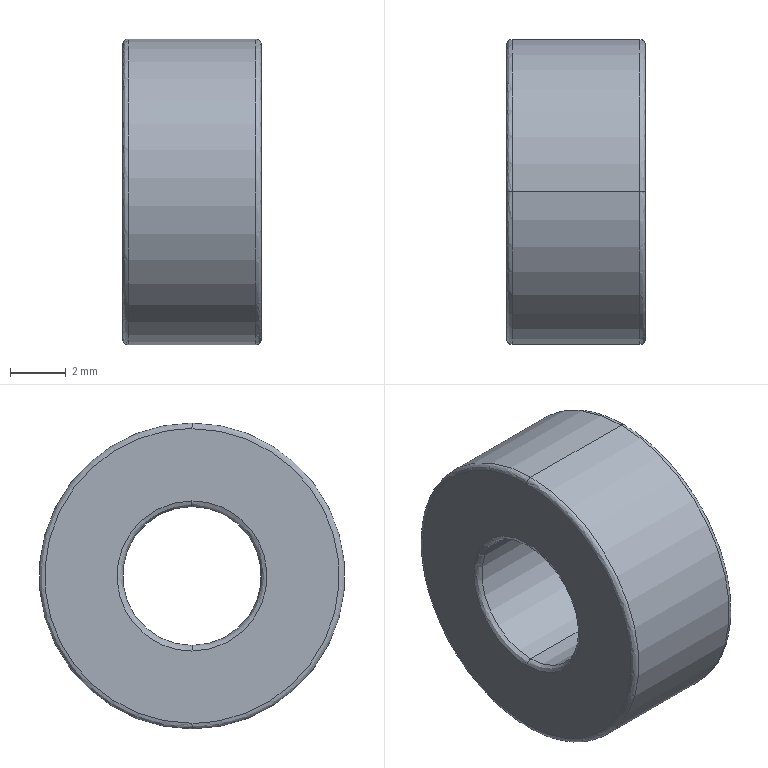Part | STEP file | Bearing B685ZZ | 1 solid | 14 faces | box 5 x 11 x 11 mm | volume 376.118 mm3 | spline 8 | cylinder 4 | plane 2 | commonest cylinder face diameters 5 x2 11 x2